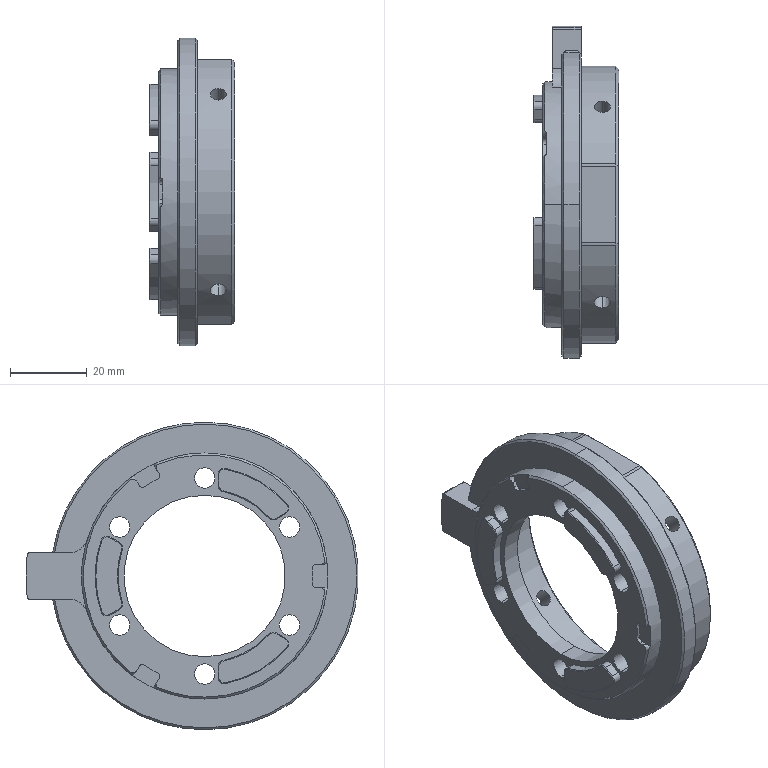NC program | NX | posted with a generic post | part box 22.3 x 86.5 x 80 mm
Lines 951 to 2662 of 3025, first 1570 of 1708 lines:
(FLOOR_WALL_2_COPY_COPY_COPY , TOOL : D2)
N1870 T18 M6
N1872 G54
N1874 G17 G0 G90 X17.592 Y-29.095 S9500 M3
N1876 G43 Z30. H18
N1878 Z-1.643
N1880 G94 G1 Z-2.643 F1000.
N1882 X16.699 Y-28.58
N1884 G3 X16.499 Y-28.58 R0.2
N1886 G2 X14.117 Y-29.828 R33.
N1888 G1 X14.015 Y-28.558
N1890 X13.875 Y-28.11
N1892 X13.705 Y-27.738
N1894 X12.733 Y-26.055
N1896 G3 X16.198 Y-24.055 R29.
N1898 G1 X17.177 Y-25.752
N1900 X17.559 Y-26.254
N1902 X17.669 Y-26.351
N1904 X17.916 Y-26.566
N1906 X18.799 Y-27.122
N1908 G2 X16.499 Y-28.58 R33.
N1910 G1 X15.999 Y-27.714
N1912 X15.997
N1914 G2 X14.976 Y-28.279 R32.
N1916 G1 X14.811 Y-27.751
N1918 X14.595 Y-27.279
N1920 X14.126 Y-26.466
N1922 G3 X15.858 Y-25.466 R30.
N1924 G1 X16.343 Y-26.307
N1926 X16.824 Y-26.94
N1928 X17.011 Y-27.104
N1930 G2 X15.999 Y-27.714 R32.
N1932 G1 X15.499 Y-26.848
N1934 G3 X15.399 Y-27.021 R0.2
N1936 G1 X16.834 Y-29.54
N1938 Z-1.643
N1940 G0 X17.592 Y-29.095 Z-1.786
N1942 G1 Z-2.786
N1944 X16.699 Y-28.58
N1946 G3 X16.499 Y-28.58 R0.2
N1948 G2 X14.117 Y-29.828 R33.
N1950 G1 X14.015 Y-28.558
N1952 X13.875 Y-28.11
N1954 X13.705 Y-27.738
N1956 X12.733 Y-26.055
N1958 G3 X16.198 Y-24.055 R29.
N1960 G1 X17.177 Y-25.752
N1962 X17.559 Y-26.254
N1964 X17.669 Y-26.351
N1966 X17.916 Y-26.566
N1968 X18.799 Y-27.122
N1970 G2 X16.499 Y-28.58 R33.
N1972 G1 X15.999 Y-27.714
N1974 X15.997
N1976 G2 X14.976 Y-28.279 R32.
N1978 G1 X14.811 Y-27.751
N1980 X14.595 Y-27.279
N1982 X14.126 Y-26.466
N1984 G3 X15.858 Y-25.466 R30.
N1986 G1 X16.343 Y-26.307
N1988 X16.824 Y-26.94
N1990 X17.011 Y-27.104
N1992 G2 X15.999 Y-27.714 R32.
N1994 G1 X15.499 Y-26.848
N1996 G3 X15.399 Y-27.021 R0.2
N1998 G1 X16.834 Y-29.54
N2000 Z-1.786
N2002 G0 X17.592 Y-29.095 Z-1.929
N2004 G1 Z-2.929
N2006 X16.699 Y-28.58
N2008 G3 X16.499 Y-28.58 R0.2
N2010 G2 X14.117 Y-29.828 R33.
N2012 G1 X14.015 Y-28.558
N2014 X13.875 Y-28.11
N2016 X13.705 Y-27.738
N2018 X12.733 Y-26.055
N2020 G3 X16.198 Y-24.055 R29.
N2022 G1 X17.177 Y-25.752
N2024 X17.559 Y-26.254
N2026 X17.669 Y-26.351
N2028 X17.916 Y-26.566
N2030 X18.799 Y-27.122
N2032 G2 X16.499 Y-28.58 R33.
N2034 G1 X15.999 Y-27.714
N2036 X15.997
N2038 G2 X14.976 Y-28.279 R32.
N2040 G1 X14.811 Y-27.751
N2042 X14.595 Y-27.279
N2044 X14.126 Y-26.466
N2046 G3 X15.858 Y-25.466 R30.
N2048 G1 X16.343 Y-26.307
N2050 X16.824 Y-26.94
N2052 X17.011 Y-27.104
N2054 G2 X15.999 Y-27.714 R32.
N2056 G1 X15.499 Y-26.848
N2058 G3 X15.399 Y-27.021 R0.2
N2060 G1 X16.834 Y-29.54
N2062 Z-1.929
N2064 G0 X17.592 Y-29.095 Z-2.071
N2066 G1 Z-3.071
N2068 X16.699 Y-28.58
N2070 G3 X16.499 Y-28.58 R0.2
N2072 G2 X14.117 Y-29.828 R33.
N2074 G1 X14.015 Y-28.558
N2076 X13.875 Y-28.11
N2078 X13.705 Y-27.738
N2080 X12.733 Y-26.055
N2082 G3 X16.198 Y-24.055 R29.
N2084 G1 X17.177 Y-25.752
N2086 X17.559 Y-26.254
N2088 X17.669 Y-26.351
N2090 X17.916 Y-26.566
N2092 X18.799 Y-27.122
N2094 G2 X16.499 Y-28.58 R33.
N2096 G1 X15.999 Y-27.714
N2098 X15.997
N2100 G2 X14.976 Y-28.279 R32.
N2102 G1 X14.811 Y-27.751
N2104 X14.595 Y-27.279
N2106 X14.126 Y-26.466
N2108 G3 X15.858 Y-25.466 R30.
N2110 G1 X16.343 Y-26.307
N2112 X16.824 Y-26.94
N2114 X17.011 Y-27.104
N2116 G2 X15.999 Y-27.714 R32.
N2118 G1 X15.499 Y-26.848
N2120 G3 X15.399 Y-27.021 R0.2
N2122 G1 X16.834 Y-29.54
N2124 Z-2.071
N2126 G0 X17.592 Y-29.095 Z-2.214
N2128 G1 Z-3.214
N2130 X16.699 Y-28.58
N2132 G3 X16.499 Y-28.58 R0.2
N2134 G2 X14.117 Y-29.828 R33.
N2136 G1 X14.015 Y-28.558
N2138 X13.875 Y-28.11
N2140 X13.705 Y-27.738
N2142 X12.733 Y-26.055
N2144 G3 X16.198 Y-24.055 R29.
N2146 G1 X17.177 Y-25.752
N2148 X17.559 Y-26.254
N2150 X17.669 Y-26.351
N2152 X17.916 Y-26.566
N2154 X18.799 Y-27.122
N2156 G2 X16.499 Y-28.58 R33.
N2158 G1 X15.999 Y-27.714
N2160 X15.997
N2162 G2 X14.976 Y-28.279 R32.
N2164 G1 X14.811 Y-27.751
N2166 X14.595 Y-27.279
N2168 X14.126 Y-26.466
N2170 G3 X15.858 Y-25.466 R30.
N2172 G1 X16.343 Y-26.307
N2174 X16.824 Y-26.94
N2176 X17.011 Y-27.104
N2178 G2 X15.999 Y-27.714 R32.
N2180 G1 X15.499 Y-26.848
N2182 G3 X15.399 Y-27.021 R0.2
N2184 G1 X16.834 Y-29.54
N2186 Z-2.214
N2188 G0 X17.592 Y-29.095 Z-2.357
N2190 G1 Z-3.357
N2192 X16.699 Y-28.58
N2194 G3 X16.499 Y-28.58 R0.2
N2196 G2 X14.117 Y-29.828 R33.
N2198 G1 X14.015 Y-28.558
N2200 X13.875 Y-28.11
N2202 X13.705 Y-27.738
N2204 X12.733 Y-26.055
N2206 G3 X16.198 Y-24.055 R29.
N2208 G1 X17.177 Y-25.752
N2210 X17.559 Y-26.254
N2212 X17.669 Y-26.351
N2214 X17.916 Y-26.566
N2216 X18.799 Y-27.122
N2218 G2 X16.499 Y-28.58 R33.
N2220 G1 X15.999 Y-27.714
N2222 X15.997
N2224 G2 X14.976 Y-28.279 R32.
N2226 G1 X14.811 Y-27.751
N2228 X14.595 Y-27.279
N2230 X14.126 Y-26.466
N2232 G3 X15.858 Y-25.466 R30.
N2234 G1 X16.343 Y-26.307
N2236 X16.824 Y-26.94
N2238 X17.011 Y-27.104
N2240 G2 X15.999 Y-27.714 R32.
N2242 G1 X15.499 Y-26.848
N2244 G3 X15.399 Y-27.021 R0.2
N2246 G1 X16.834 Y-29.54
N2248 Z-2.357
N2250 G0 X17.592 Y-29.095 Z-2.5
N2252 G1 Z-3.5
N2254 X16.699 Y-28.58
N2256 G3 X16.499 Y-28.58 R0.2
N2258 G2 X14.117 Y-29.828 R33.
N2260 G1 X14.015 Y-28.558
N2262 X13.875 Y-28.11
N2264 X13.705 Y-27.738
N2266 X12.733 Y-26.055
N2268 G3 X16.198 Y-24.055 R29.
N2270 G1 X17.177 Y-25.752
N2272 X17.559 Y-26.254
N2274 X17.669 Y-26.351
N2276 X17.916 Y-26.566
N2278 X18.799 Y-27.122
N2280 G2 X16.499 Y-28.58 R33.
N2282 G1 X15.999 Y-27.714
N2284 X15.997
N2286 G2 X14.976 Y-28.279 R32.
N2288 G1 X14.811 Y-27.751
N2290 X14.595 Y-27.279
N2292 X14.126 Y-26.466
N2294 G3 X15.858 Y-25.466 R30.
N2296 G1 X16.343 Y-26.307
N2298 X16.824 Y-26.94
N2300 X17.011 Y-27.104
N2302 G2 X15.999 Y-27.714 R32.
N2304 G1 X15.499 Y-26.848
N2306 G3 X15.399 Y-27.021 R0.2
N2308 G1 X16.834 Y-29.54
N2310 Z-2.5
N2312 G0 Z30.
N2314 X16.401 Y29.782
N2316 Z-1.643
N2318 G1 Z-2.643
N2320 Y28.751
N2322 G3 X16.501 Y28.578 R0.2
N2324 G2 X18.774 Y27.139 R33.
N2326 G1 X17.725 Y26.417
N2328 X17.406 Y26.071
N2330 X17.169 Y25.738
N2332 X16.198 Y24.055
N2334 G3 X12.733 Y26.055 R29.
N2336 G1 X13.713 Y27.752
N2338 X13.957 Y28.334
N2340 X13.986 Y28.478
N2342 X14.049 Y28.799
N2344 X14.089 Y29.841
N2346 G2 X16.501 Y28.578 R33.
N2348 G1 X16.001 Y27.712
N2350 X16.003 Y27.711
N2352 G2 X17.003 Y27.109 R32.
N2354 G1 X16.628 Y26.702
N2356 X16.327 Y26.279
N2358 X15.858 Y25.466
N2360 G3 X14.126 Y26.466 R30.
N2362 G1 X14.611 Y27.307
N2364 X14.919 Y28.041
N2366 X14.967 Y28.284
N2368 G2 X16.001 Y27.712 R32.
N2370 G1 X15.501 Y26.846
N2372 G3 X15.701 Y26.846 R0.2
N2374 G1 X17.165 Y29.349
N2376 Z-1.643
N2378 G0 X16.401 Y29.782 Z-1.786
N2380 G1 Z-2.786
N2382 Y28.751
N2384 G3 X16.501 Y28.578 R0.2
N2386 G2 X18.774 Y27.139 R33.
N2388 G1 X17.725 Y26.417
N2390 X17.406 Y26.071
N2392 X17.169 Y25.738
N2394 X16.198 Y24.055
N2396 G3 X12.733 Y26.055 R29.
N2398 G1 X13.713 Y27.752
N2400 X13.957 Y28.334
N2402 X13.986 Y28.478
N2404 X14.049 Y28.799
N2406 X14.089 Y29.841
N2408 G2 X16.501 Y28.578 R33.
N2410 G1 X16.001 Y27.712
N2412 X16.003 Y27.711
N2414 G2 X17.003 Y27.109 R32.
N2416 G1 X16.628 Y26.702
N2418 X16.327 Y26.279
N2420 X15.858 Y25.466
N2422 G3 X14.126 Y26.466 R30.
N2424 G1 X14.611 Y27.307
N2426 X14.919 Y28.041
N2428 X14.967 Y28.284
N2430 G2 X16.001 Y27.712 R32.
N2432 G1 X15.501 Y26.846
N2434 G3 X15.701 Y26.846 R0.2
N2436 G1 X17.165 Y29.349
N2438 Z-1.786
N2440 G0 X16.401 Y29.782 Z-1.929
N2442 G1 Z-2.929
N2444 Y28.751
N2446 G3 X16.501 Y28.578 R0.2
N2448 G2 X18.774 Y27.139 R33.
N2450 G1 X17.725 Y26.417
N2452 X17.406 Y26.071
N2454 X17.169 Y25.738
N2456 X16.198 Y24.055
N2458 G3 X12.733 Y26.055 R29.
N2460 G1 X13.713 Y27.752
N2462 X13.957 Y28.334
N2464 X13.986 Y28.478
N2466 X14.049 Y28.799
N2468 X14.089 Y29.841
N2470 G2 X16.501 Y28.578 R33.
N2472 G1 X16.001 Y27.712
N2474 X16.003 Y27.711
N2476 G2 X17.003 Y27.109 R32.
N2478 G1 X16.628 Y26.702
N2480 X16.327 Y26.279
N2482 X15.858 Y25.466
N2484 G3 X14.126 Y26.466 R30.
N2486 G1 X14.611 Y27.307
N2488 X14.919 Y28.041
N2490 X14.967 Y28.284
N2492 G2 X16.001 Y27.712 R32.
N2494 G1 X15.501 Y26.846
N2496 G3 X15.701 Y26.846 R0.2
N2498 G1 X17.165 Y29.349
N2500 Z-1.929
N2502 G0 X16.401 Y29.782 Z-2.071
N2504 G1 Z-3.071
N2506 Y28.751
N2508 G3 X16.501 Y28.578 R0.2
N2510 G2 X18.774 Y27.139 R33.
N2512 G1 X17.725 Y26.417
N2514 X17.406 Y26.071
N2516 X17.169 Y25.738
N2518 X16.198 Y24.055
N2520 G3 X12.733 Y26.055 R29.
N2522 G1 X13.713 Y27.752
N2524 X13.957 Y28.334
N2526 X13.986 Y28.478
N2528 X14.049 Y28.799
N2530 X14.089 Y29.841
N2532 G2 X16.501 Y28.578 R33.
N2534 G1 X16.001 Y27.712
N2536 X16.003 Y27.711
N2538 G2 X17.003 Y27.109 R32.
N2540 G1 X16.628 Y26.702
N2542 X16.327 Y26.279
N2544 X15.858 Y25.466
N2546 G3 X14.126 Y26.466 R30.
N2548 G1 X14.611 Y27.307
N2550 X14.919 Y28.041
N2552 X14.967 Y28.284
N2554 G2 X16.001 Y27.712 R32.
N2556 G1 X15.501 Y26.846
N2558 G3 X15.701 Y26.846 R0.2
N2560 G1 X17.165 Y29.349
N2562 Z-2.071
N2564 G0 X16.401 Y29.782 Z-2.214
N2566 G1 Z-3.214
N2568 Y28.751
N2570 G3 X16.501 Y28.578 R0.2
N2572 G2 X18.774 Y27.139 R33.
N2574 G1 X17.725 Y26.417
N2576 X17.406 Y26.071
N2578 X17.169 Y25.738
N2580 X16.198 Y24.055
N2582 G3 X12.733 Y26.055 R29.
N2584 G1 X13.713 Y27.752
N2586 X13.957 Y28.334
N2588 X13.986 Y28.478
N2590 X14.049 Y28.799
N2592 X14.089 Y29.841
N2594 G2 X16.501 Y28.578 R33.
N2596 G1 X16.001 Y27.712
N2598 X16.003 Y27.711
N2600 G2 X17.003 Y27.109 R32.
N2602 G1 X16.628 Y26.702
N2604 X16.327 Y26.279
N2606 X15.858 Y25.466
N2608 G3 X14.126 Y26.466 R30.
N2610 G1 X14.611 Y27.307
N2612 X14.919 Y28.041
N2614 X14.967 Y28.284
N2616 G2 X16.001 Y27.712 R32.
N2618 G1 X15.501 Y26.846
N2620 G3 X15.701 Y26.846 R0.2
N2622 G1 X17.165 Y29.349
N2624 Z-2.214
N2626 G0 X16.401 Y29.782 Z-2.357
N2628 G1 Z-3.357
N2630 Y28.751
N2632 G3 X16.501 Y28.578 R0.2
N2634 G2 X18.774 Y27.139 R33.
N2636 G1 X17.725 Y26.417
N2638 X17.406 Y26.071
N2640 X17.169 Y25.738
N2642 X16.198 Y24.055
N2644 G3 X12.733 Y26.055 R29.
N2646 G1 X13.713 Y27.752
N2648 X13.957 Y28.334
N2650 X13.986 Y28.478
N2652 X14.049 Y28.799
N2654 X14.089 Y29.841
N2656 G2 X16.501 Y28.578 R33.
N2658 G1 X16.001 Y27.712
N2660 X16.003 Y27.711
N2662 G2 X17.003 Y27.109 R32.
N2664 G1 X16.628 Y26.702
N2666 X16.327 Y26.279
N2668 X15.858 Y25.466
N2670 G3 X14.126 Y26.466 R30.
N2672 G1 X14.611 Y27.307
N2674 X14.919 Y28.041
N2676 X14.967 Y28.284
N2678 G2 X16.001 Y27.712 R32.
N2680 G1 X15.501 Y26.846
N2682 G3 X15.701 Y26.846 R0.2
N2684 G1 X17.165 Y29.349
N2686 Z-2.357
N2688 G0 X16.401 Y29.782 Z-2.5
N2690 G1 Z-3.5
N2692 Y28.751
N2694 G3 X16.501 Y28.578 R0.2
N2696 G2 X18.774 Y27.139 R33.
N2698 G1 X17.725 Y26.417
N2700 X17.406 Y26.071
N2702 X17.169 Y25.738
N2704 X16.198 Y24.055
N2706 G3 X12.733 Y26.055 R29.
N2708 G1 X13.713 Y27.752
N2710 X13.957 Y28.334
N2712 X13.986 Y28.478
N2714 X14.049 Y28.799
N2716 X14.089 Y29.841
N2718 G2 X16.501 Y28.578 R33.
N2720 G1 X16.001 Y27.712
N2722 X16.003 Y27.711
N2724 G2 X17.003 Y27.109 R32.
N2726 G1 X16.628 Y26.702
N2728 X16.327 Y26.279
N2730 X15.858 Y25.466
N2732 G3 X14.126 Y26.466 R30.
N2734 G1 X14.611 Y27.307
N2736 X14.919 Y28.041
N2738 X14.967 Y28.284
N2740 G2 X16.001 Y27.712 R32.
N2742 G1 X15.501 Y26.846
N2744 G3 X15.701 Y26.846 R0.2
N2746 G1 X17.165 Y29.349
N2748 Z-2.5
N2750 G0 Z30.
N2752 X-33.993 Y-0.687
N2754 Z-1.643
N2756 G1 Z-2.643
N2758 X-33.1 Y-0.172
N2760 G3 X-33. Y0.002 R0.2
N2762 G2 X-32.89 Y2.689 R33.
N2764 G1 X-31.74 Y2.142
N2766 X-31.281 Y2.038
N2768 X-30.874 Y2.
N2770 X-28.931
N2772 G3 X-28.931 Y-2. R29.
N2774 G1 X-30.891
N2776 X-31.517 Y-2.079
N2778 X-31.655 Y-2.127
N2780 X-31.965 Y-2.233
N2782 X-32.888 Y-2.719
N2784 G2 X-33. Y0.002 R33.
N2786 G1 X-32.
N2788 Y0.003
N2790 G2 X-31.979 Y1.17 R32.
N2792 G1 X-31.439 Y1.049
N2794 X-30.921 Y1.
N2796 X-29.983
N2798 G3 X-29.983 Y-1. R30.
N2800 G1 X-30.954
N2802 X-31.743 Y-1.1
N2804 X-31.978 Y-1.18
N2806 G2 X-32. Y0.002 R32.
N2808 G1 X-31. Y0.001
N2810 G3 X-31.1 Y0.175 R0.2
N2812 G1 X-33.999 Y0.191
N2814 Z-1.643
N2816 G0 X-33.993 Y-0.687 Z-1.786
N2818 G1 Z-2.786
N2820 X-33.1 Y-0.172
N2822 G3 X-33. Y0.002 R0.2
N2824 G2 X-32.89 Y2.689 R33.
N2826 G1 X-31.74 Y2.142
N2828 X-31.281 Y2.038
N2830 X-30.874 Y2.
N2832 X-28.931
N2834 G3 X-28.931 Y-2. R29.
N2836 G1 X-30.891
N2838 X-31.517 Y-2.079
N2840 X-31.655 Y-2.127
N2842 X-31.965 Y-2.233
N2844 X-32.888 Y-2.719
N2846 G2 X-33. Y0.002 R33.
N2848 G1 X-32.
N2850 Y0.003
N2852 G2 X-31.979 Y1.17 R32.
N2854 G1 X-31.439 Y1.049
N2856 X-30.921 Y1.
N2858 X-29.983
N2860 G3 X-29.983 Y-1. R30.
N2862 G1 X-30.954
N2864 X-31.743 Y-1.1
N2866 X-31.978 Y-1.18
N2868 G2 X-32. Y0.002 R32.
N2870 G1 X-31. Y0.001
N2872 G3 X-31.1 Y0.175 R0.2
N2874 G1 X-33.999 Y0.191
N2876 Z-1.786
N2878 G0 X-33.993 Y-0.687 Z-1.929
N2880 G1 Z-2.929
N2882 X-33.1 Y-0.172
N2884 G3 X-33. Y0.002 R0.2
N2886 G2 X-32.89 Y2.689 R33.
N2888 G1 X-31.74 Y2.142
N2890 X-31.281 Y2.038
N2892 X-30.874 Y2.
N2894 X-28.931
N2896 G3 X-28.931 Y-2. R29.
N2898 G1 X-30.891
N2900 X-31.517 Y-2.079
N2902 X-31.655 Y-2.127
N2904 X-31.965 Y-2.233
N2906 X-32.888 Y-2.719
N2908 G2 X-33. Y0.002 R33.
N2910 G1 X-32.
N2912 Y0.003
N2914 G2 X-31.979 Y1.17 R32.
N2916 G1 X-31.439 Y1.049
N2918 X-30.921 Y1.
N2920 X-29.983
N2922 G3 X-29.983 Y-1. R30.
N2924 G1 X-30.954
N2926 X-31.743 Y-1.1
N2928 X-31.978 Y-1.18
N2930 G2 X-32. Y0.002 R32.
N2932 G1 X-31. Y0.001
N2934 G3 X-31.1 Y0.175 R0.2
N2936 G1 X-33.999 Y0.191
N2938 Z-1.929
N2940 G0 X-33.993 Y-0.687 Z-2.071
N2942 G1 Z-3.071
N2944 X-33.1 Y-0.172
N2946 G3 X-33. Y0.002 R0.2
N2948 G2 X-32.89 Y2.689 R33.
N2950 G1 X-31.74 Y2.142
N2952 X-31.281 Y2.038
N2954 X-30.874 Y2.
N2956 X-28.931
N2958 G3 X-28.931 Y-2. R29.
N2960 G1 X-30.891
N2962 X-31.517 Y-2.079
N2964 X-31.655 Y-2.127
N2966 X-31.965 Y-2.233
N2968 X-32.888 Y-2.719
N2970 G2 X-33. Y0.002 R33.
N2972 G1 X-32.
N2974 Y0.003
N2976 G2 X-31.979 Y1.17 R32.
N2978 G1 X-31.439 Y1.049
N2980 X-30.921 Y1.
N2982 X-29.983
N2984 G3 X-29.983 Y-1. R30.
N2986 G1 X-30.954
N2988 X-31.743 Y-1.1
N2990 X-31.978 Y-1.18
N2992 G2 X-32. Y0.002 R32.
N2994 G1 X-31. Y0.001
N2996 G3 X-31.1 Y0.175 R0.2
N2998 G1 X-33.999 Y0.191
N3000 Z-2.071
N3002 G0 X-33.993 Y-0.687 Z-2.214
N3004 G1 Z-3.214
N3006 X-33.1 Y-0.172
N3008 G3 X-33. Y0.002 R0.2
N3010 G2 X-32.89 Y2.689 R33.
N3012 G1 X-31.74 Y2.142
N3014 X-31.281 Y2.038
N3016 X-30.874 Y2.
N3018 X-28.931
N3020 G3 X-28.931 Y-2. R29.
N3022 G1 X-30.891
N3024 X-31.517 Y-2.079
N3026 X-31.655 Y-2.127
N3028 X-31.965 Y-2.233
N3030 X-32.888 Y-2.719
N3032 G2 X-33. Y0.002 R33.
N3034 G1 X-32.
N3036 Y0.003
N3038 G2 X-31.979 Y1.17 R32.
N3040 G1 X-31.439 Y1.049
N3042 X-30.921 Y1.
N3044 X-29.983
N3046 G3 X-29.983 Y-1. R30.
N3048 G1 X-30.954
N3050 X-31.743 Y-1.1
N3052 X-31.978 Y-1.18
N3054 G2 X-32. Y0.002 R32.
N3056 G1 X-31. Y0.001
N3058 G3 X-31.1 Y0.175 R0.2
N3060 G1 X-33.999 Y0.191
N3062 Z-2.214
N3064 G0 X-33.993 Y-0.687 Z-2.357
N3066 G1 Z-3.357
N3068 X-33.1 Y-0.172
N3070 G3 X-33. Y0.002 R0.2
N3072 G2 X-32.89 Y2.689 R33.
N3074 G1 X-31.74 Y2.142
N3076 X-31.281 Y2.038
N3078 X-30.874 Y2.
N3080 X-28.931
N3082 G3 X-28.931 Y-2. R29.
N3084 G1 X-30.891
N3086 X-31.517 Y-2.079
N3088 X-31.655 Y-2.127
N3090 X-31.965 Y-2.233
N3092 X-32.888 Y-2.719
N3094 G2 X-33. Y0.002 R33.
N3096 G1 X-32.
N3098 Y0.003
N3100 G2 X-31.979 Y1.17 R32.
N3102 G1 X-31.439 Y1.049
N3104 X-30.921 Y1.
N3106 X-29.983
N3108 G3 X-29.983 Y-1. R30.
N3110 G1 X-30.954
N3112 X-31.743 Y-1.1
N3114 X-31.978 Y-1.18
N3116 G2 X-32. Y0.002 R32.
N3118 G1 X-31. Y0.001
N3120 G3 X-31.1 Y0.175 R0.2
N3122 G1 X-33.999 Y0.191
N3124 Z-2.357
N3126 G0 X-33.993 Y-0.687 Z-2.5
N3128 G1 Z-3.5
N3130 X-33.1 Y-0.172
N3132 G3 X-33. Y0.002 R0.2
N3134 G2 X-32.89 Y2.689 R33.
N3136 G1 X-31.74 Y2.142
N3138 X-31.281 Y2.038
N3140 X-30.874 Y2.
N3142 X-28.931
N3144 G3 X-28.931 Y-2. R29.
N3146 G1 X-30.891
N3148 X-31.517 Y-2.079
N3150 X-31.655 Y-2.127
N3152 X-31.965 Y-2.233
N3154 X-32.888 Y-2.719
N3156 G2 X-33. Y0.002 R33.
N3158 G1 X-32.
N3160 Y0.003
N3162 G2 X-31.979 Y1.17 R32.
N3164 G1 X-31.439 Y1.049
N3166 X-30.921 Y1.
N3168 X-29.983
N3170 G3 X-29.983 Y-1. R30.
N3172 G1 X-30.954
N3174 X-31.743 Y-1.1
N3176 X-31.978 Y-1.18
N3178 G2 X-32. Y0.002 R32.
N3180 G1 X-31. Y0.001
N3182 G3 X-31.1 Y0.175 R0.2
N3184 G1 X-33.999 Y0.191
N3186 Z-2.5
N3188 G0 Z30.
(ZLEVEL_PROFILE_1_COPY , TOOL : D2)
N3190 X13.293 Y-26.223
N3192 Z-1.035
N3194 G1 Z-2.535 F1500.
N3196 X12.905 Y-26.156
N3198 G3 X12.907 Y-26.356 R0.2
N3200 G2 X13.255 Y-26.971 R17.468
N3202 X13.543 Y-28.664 R2.678
N3204 X12.415 Y-30.075 R1.83
N3206 G1 X11.91 Y-30.277
N3208 Y-30.315 Z-2.571
N3210 X12.464 Y-30.09
N3212 G3 X13.534 Y-28.822 R1.779
N3214 X13.308 Y-27.066 R2.629
N3216 G1 X12.907 Y-26.356
N3218 Z-2.606
N3220 X13.273 Y-27.001
N3222 G2 X13.555 Y-28.835 R2.609
N3224 X12.508 Y-30.111 R1.801
N3226 G1 X11.91 Y-30.353
N3228 Y-30.391 Z-2.641
N3230 X12.508 Y-30.149
N3232 G3 X13.578 Y-28.84 R1.804
N3234 X13.312 Y-27.066 R2.651
N3236 G1 X12.907 Y-26.356
N3238 Z-2.676
N3240 X13.315 Y-27.066
N3242 G2 X13.624 Y-28.723 R2.713
N3244 X12.486 Y-30.197 R1.853
N3246 G1 X12.109 Y-30.35
N3248 Y-30.388 Z-2.712
N3250 X12.508 Y-30.226
N3252 G3 X13.655 Y-28.643 R1.838
N3254 X13.316 Y-27.066 R2.772
N3256 G1 X12.907 Y-26.356
N3258 Z-2.747
N3260 G2 X13.413 Y-27.264 R14.43
N3262 X13.603 Y-29.041 R2.535
N3264 X12.649 Y-30.2 R1.779
N3266 G1 X12.608 Y-30.219
N3268 X12.133 Y-30.416
N3270 X12.109 Y-30.464 Z-2.782
N3272 G3 X12.713 Y-30.204 R4.238
N3274 X13.669 Y-28.877 R1.832
N3276 X13.416 Y-27.264 R2.616
N3278 X12.907 Y-26.356 R18.367
N3280 G1 X12.976 Y-26.475 Z-2.818
N3282 G2 X13.419 Y-27.264 R17.197
N3284 X13.663 Y-29.011 R2.591
N3286 X12.568 Y-30.317 R1.813
N3288 G1 X12.109 Y-30.502
N3290 Y-30.54 Z-2.853
N3292 X12.577 Y-30.351
N3294 G3 X13.707 Y-28.926 R1.839
N3296 X13.422 Y-27.264 R2.661
N3298 X12.976 Y-26.475 R23.63
N3300 G1 Z-2.888
N3302 X13.425 Y-27.264
N3304 X13.506 Y-27.424
N3306 G2 X13.713 Y-29.015 R2.653
N3308 X12.605 Y-30.378 R1.815
N3310 G1 X12.109 Y-30.578
N3312 X12.115 Y-30.613 Z-2.924
N3314 X12.656 Y-30.392
N3316 G3 X13.616 Y-29.419 R1.743
N3318 X13.753 Y-28.249 R2.294
N3320 X13.428 Y-27.264 R2.927
N3322 G1 X12.976 Y-26.475
N3324 Z-2.959
N3326 X13.43 Y-27.264
N3328 G2 X13.705 Y-27.942 R3.263
N3330 X13.714 Y-29.219 R2.526
N3332 X12.804 Y-30.361 R1.773
N3334 X12.211 Y-30.613 R4.489
N3336 G1 X12.16 Y-30.653 Z-2.976
N3338 X12.109 Y-30.692 Z-2.994
N3340 X12.708 Y-30.449
N3342 G3 X13.705 Y-29.342 R1.786
N3344 X13.705 Y-27.912 R2.486
N3346 X13.431 Y-27.264 R3.303
N3348 G1 X12.976 Y-26.475
N3350 Z-3.029
N3352 X13.506 Y-27.402
N3354 X13.531 Y-27.461
N3356 X13.585 Y-27.576
N3358 G2 X13.757 Y-29.248 R2.557
N3360 X12.748 Y-30.46 R1.766
N3362 G1 X12.303 Y-30.655
N3364 X12.322 Y-30.685 Z-3.065
N3366 X12.755 Y-30.497
N3368 G3 X13.78 Y-29.261 R1.78
N3370 X13.615 Y-27.639 R2.551
N3372 G1 X13.506 Y-27.398
N3374 X13.107 Y-26.701
N3376 Z-3.1
N3378 X13.506 Y-27.395
N3380 X13.603 Y-27.598
N3382 G2 X13.806 Y-29.258 R2.602
N3384 X12.767 Y-30.531 R1.784
N3386 G1 X12.34 Y-30.715
N3388 X12.359 Y-30.745 Z-3.135
N3390 G3 X12.897 Y-30.509 R3.901
N3392 X13.863 Y-29.081 R1.842
N3394 X13.54 Y-27.461 R2.759
N3396 G1 X13.506 Y-27.393
N3398 X13.107 Y-26.701
N3400 Z-3.17
N3402 X13.543 Y-27.461
N3404 G2 X13.902 Y-28.84 R2.931
N3406 X13.107 Y-30.432 R1.944
N3408 X12.377 Y-30.776 R4.073
N3410 G1 X12.396 Y-30.807 Z-3.206
N3412 G3 X13.306 Y-30.318 R2.886
N3414 X13.912 Y-28.643 R2.032
N3416 X13.544 Y-27.461 R3.002
N3418 G1 X13.107 Y-26.701
N3420 Z-3.241
N3422 G2 X13.643 Y-27.658 R16.017
N3424 X13.903 Y-29.271 R2.634
N3426 X12.931 Y-30.613 R1.825
N3428 X12.436 Y-30.827 R4.263
N3430 G1 X12.479 Y-30.848 Z-3.276
N3432 X13.016 Y-30.611
N3434 G3 X13.906 Y-29.367 R1.809
N3436 X13.646 Y-27.658 R2.626
N3438 X13.204 Y-26.869 R16.196
N3440 G1 Z-3.311
N3442 G2 X13.65 Y-27.658 R20.176
N3444 X13.952 Y-29.234 R2.687
N3446 X12.586 Y-30.841 R1.894
N3448 G1 X12.67 Y-30.821 Z-3.323
N3450 X12.753 Y-30.799 Z-3.335
N3452 X12.835 Y-30.774 Z-3.347
N3454 G3 X13.941 Y-29.431 R1.801
N3456 X13.705 Y-27.754 R2.705
N3458 X13.204 Y-26.869 R29.664
N3460 G1 Z-3.382
N3462 X13.656 Y-27.658
N3464 X13.705 Y-27.75
N3466 G2 X13.965 Y-29.431 R2.677
N3468 X13.169 Y-30.644 R1.839
N3470 G1 X13.239 Y-30.614 Z-3.394
N3472 X13.307 Y-30.578 Z-3.406
N3474 X13.368 Y-30.535 Z-3.417
N3476 G3 X13.989 Y-29.431 R1.827
N3478 X13.705 Y-27.747 R2.675
N3480 G1 X13.658 Y-27.658
N3482 X13.204 Y-26.869
N3484 Z-3.453
N3486 X13.659 Y-27.658
N3488 X13.705 Y-27.744
N3490 G2 X14.038 Y-29.234 R2.746
N3492 X13.524 Y-30.443 R1.972
N3494 G1 X13.582 Y-30.406 Z-3.472
N3496 X13.634 Y-30.365 Z-3.49
N3498 G3 X14.06 Y-29.234 R1.973
N3500 X13.705 Y-27.74 R2.754
N3502 G1 X13.659 Y-27.658
N3504 X13.317 Y-27.066
N3506 Z-3.5
N3508 X13.659 Y-27.658
N3510 X13.705 Y-27.739
N3512 G2 X14.064 Y-29.234 R2.76
N3514 X13.655 Y-30.35 R1.984
N3516 G3 X13.629 Y-30.548 R0.2
N3518 G1 X13.745 Y-30.83
N3520 Z-2.
N3522 G0 Z30.
N3524 X20.79 Y-25.544
N3526 Z-1.035
N3528 G1 Z-2.535
N3530 X20.248 Y-25.497
N3532 X20.211 Y-25.49
N3534 X20.176 Y-25.506
N3536 X20.157 Y-25.539
N3538 X20.15 Y-25.549
N3540 X19.706 Y-25.884
N3542 X19.689 Y-25.896
N3544 G2 X17.894 Y-25.997 R1.851
N3546 X16.697 Y-24.916 R2.733
N3548 G1 X16.343 Y-24.308
N3550 Z-2.571
N3552 X16.686 Y-24.899
N3554 G3 X17.94 Y-26.041 R2.752
N3556 X19.71 Y-25.918 R1.866
N3558 X20.17 Y-25.574 R3.709
N3560 G1 X20.182 Y-25.591 Z-2.588
N3562 X20.191 Y-25.602 Z-2.606
N3564 G2 X19.489 Y-26.087 R3.67
N3566 X17.894 Y-26.043 R1.893
N3568 X16.813 Y-25.096 R2.664
N3570 X16.343 Y-24.308 R15.612
N3572 G1 Z-2.641
N3574 G3 X16.81 Y-25.096 R18.778
N3576 X17.894 Y-26.066 R2.68
N3578 X19.489 Y-26.125 R1.899
N3580 X20.212 Y-25.631 R3.572
N3582 G1 X20.224 Y-25.666 Z-2.676
N3584 G2 X19.706 Y-26.045 R3.413
N3586 X17.92 Y-26.102 R1.843
N3588 G1 X17.88 Y-26.081
N3590 G2 X16.807 Y-25.096 R2.697
N3592 G1 X16.343 Y-24.308
N3594 Z-2.712
N3596 X16.804 Y-25.096
N3598 G3 X17.838 Y-26.081 R2.727
N3600 G1 X17.942 Y-26.135
N3602 G3 X19.702 Y-26.089 R1.836
N3604 X20.252 Y-25.689 R3.297
N3606 G1 X20.263 Y-25.708 Z-2.729
N3608 X20.27 Y-25.72 Z-2.747
N3610 G2 X19.489 Y-26.241 R3.151
N3612 X17.894 Y-26.131 R1.924
N3614 X16.801 Y-25.096 R2.754
N3616 G1 X16.343 Y-24.308
N3618 Z-2.782
N3620 X16.799 Y-25.096
N3622 G3 X18.095 Y-26.248 R2.755
N3624 X19.73 Y-26.155 R1.832
N3626 X20.287 Y-25.751 R3.233
N3628 G1 X20.301 Y-25.785 Z-2.818
N3630 G2 X19.842 Y-26.129 R4.355
N3632 X18.118 Y-26.282 R1.843
N3634 X16.927 Y-25.293 R2.685
N3636 X16.343 Y-24.308 R20.422
N3638 G1 X16.457 Y-24.505 Z-2.853
N3640 G3 X16.896 Y-25.25 R21.125
N3642 X18.125 Y-26.306 R2.674
N3644 X19.876 Y-26.151 R1.867
N3646 X20.318 Y-25.816 R4.014
N3648 G1 X20.329 Y-25.835 Z-2.871
N3650 X20.335 Y-25.848 Z-2.888
N3652 X20.327 Y-25.859
N3654 X19.965 Y-26.131
N3656 G2 X18.311 Y-26.397 R1.793
N3658 X16.921 Y-25.293 R2.627
N3660 G1 X16.896 Y-25.254
N3662 X16.457 Y-24.505
N3664 X16.497 Y-24.574 Z-2.924
N3666 X16.571 Y-24.702
N3668 X16.896 Y-25.259
N3670 X16.964 Y-25.363
N3672 G3 X18.318 Y-26.424 R2.623
N3674 X19.988 Y-26.156 R1.797
N3676 G1 X20.346 Y-25.884
N3678 X20.403 Z-2.959
N3680 X19.888 Y-26.275
N3682 G2 X18.093 Y-26.361 R1.856
N3684 X17.052 Y-25.49 R2.622
N3686 G1 X16.916 Y-25.293
N3688 X16.896 Y-25.263
N3690 X16.497 Y-24.574
N3692 Z-2.994
N3694 X16.896 Y-25.265
N3696 X16.913 Y-25.293
N3698 G3 X17.894 Y-26.281 R2.881
N3700 X19.689 Y-26.425 R1.965
N3702 X20.46 Y-25.884 R4.309
N3704 G1 X20.426 Y-25.937 Z-3.012
N3706 X20.387 Y-25.986 Z-3.029
N3708 G2 X19.689 Y-26.464 R3.466
N3710 X18.126 Y-26.422 R1.903
N3712 X17.002 Y-25.425 R2.763
N3714 X16.497 Y-24.574 R14.283
N3716 G1 X16.571 Y-24.702 Z-3.065
N3718 G3 X17.036 Y-25.484 R13.382
N3720 X17.999 Y-26.377 R2.629
N3722 G1 X18.087 Y-26.424
N3724 G3 X19.901 Y-26.386 R1.837
N3726 X20.406 Y-26.016 R3.363
N3728 G1 X20.423 Y-26.03 Z-3.082
N3730 X20.435 Y-26.04 Z-3.1
N3732 X19.888 Y-26.441
N3734 G2 X18.133 Y-26.47 R1.867
N3736 X17.042 Y-25.497 R2.664
N3738 X16.571 Y-24.702 R15.232
N3740 G1 Z-3.135
N3742 G3 X17.038 Y-25.495 R23.231
N3744 X18.219 Y-26.528 R2.647
N3746 G1 X18.293 Y-26.561
N3748 G3 X19.901 Y-26.475 R1.844
N3750 G1 X20.464 Y-26.063
N3752 X20.465 Y-26.108 Z-3.17
N3754 X19.966 Y-26.475
N3756 G2 X18.399 Y-26.627 R1.805
N3758 X17.031 Y-25.49 R2.679
N3760 G1 X16.571 Y-24.702
N3762 Z-3.206
N3764 X17.028 Y-25.49
N3766 G3 X18.33 Y-26.625 R2.713
N3768 X20.057 Y-26.455 R1.842
N3770 X20.482 Y-26.14 R5.299
N3772 G1 X20.542 Y-26.131 Z-3.241
N3774 G2 X20.074 Y-26.487 R4.453
N3776 X18.344 Y-26.654 R1.855
N3778 X17.096 Y-25.597 R2.666
N3780 G1 X17.027 Y-25.49
N3782 X16.571 Y-24.702
N3784 Z-3.276
N3786 X17.026 Y-25.49
N3788 X17.096 Y-25.601
N3790 G3 X18.331 Y-26.673 R2.702
N3792 X20.085 Y-26.522 R1.858
N3794 X20.567 Y-26.153 R4.099
N3796 G1 X20.508 Y-26.223 Z-3.288
N3798 X20.444 Y-26.287 Z-3.3
N3800 X20.379 Y-26.35 Z-3.311
N3802 G2 X18.279 Y-26.672 R1.88
N3804 X17.151 Y-25.687 R2.685
N3806 G1 X17.096 Y-25.604
N3808 X16.685 Y-24.899
N3810 X16.697 Y-24.92 Z-3.347
N3812 X17.096 Y-25.608
N3814 X17.148 Y-25.687
N3816 G3 X18.492 Y-26.781 R2.668
N3818 X20.229 Y-26.506 R1.808
N3820 G1 X20.167 Y-26.567 Z-3.355
N3822 X20.1 Y-26.623 Z-3.364
N3824 X20.032 Y-26.677 Z-3.373
N3826 X19.959 Y-26.723 Z-3.382
N3828 G2 X18.492 Y-26.806 R1.832
N3830 X17.145 Y-25.687 R2.676
N3832 G1 X17.096 Y-25.61
N3834 X16.697 Y-24.92
N3836 Z-3.417
N3838 X17.096 Y-25.611
N3840 X17.142 Y-25.687
N3842 G3 X18.492 Y-26.831 R2.712
N3844 X19.754 Y-26.85 R1.87
N3846 G1 X19.683 Y-26.896 Z-3.435
N3848 X19.608 Y-26.928 Z-3.453
N3850 G2 X18.293 Y-26.771 R1.927
N3852 X17.141 Y-25.687 R2.786
N3854 G1 X17.096 Y-25.611
N3856 X16.697 Y-24.92
N3858 Z-3.49
N3860 X17.14 Y-25.687
N3862 G3 X18.293 Y-26.794 R2.781
N3864 X19.48 Y-26.993 R2.001
N3866 G1 X19.457 Y-27.001 Z-3.5
N3868 G2 X18.293 Y-26.799 R1.975
N3870 X17.14 Y-25.687 R2.783
N3872 G1 X16.697 Y-24.92
N3874 G3 X16.524 Y-24.82 R0.2
N3876 G1 X16.177
N3878 Z-2.
N3880 G0 Z30.
N3882 X-29.356 Y1.6
N3884 Z-1.035
N3886 G1 Z-2.535
N3888 X-29.098 Y1.9
N3890 G3 X-29.271 Y2. R0.2
N3892 G1 X-29.944 Y2.002
N3894 X-30.004 Y2.004
N3896 G2 X-31.669 Y2.665 R2.645
N3898 X-32.253 Y4.211 R1.768
N3900 G1 X-32.175 Y4.827
N3902 X-32.215 Y4.799 Z-2.571
N3904 G3 X-32.301 Y4.094 R4.122
N3906 X-31.495 Y2.493 R1.864
N3908 X-29.868 Y2. R2.796
N3910 G1 X-29.271
N3912 Z-2.606
N3914 X-29.919
N3916 G2 X-31.26 Y2.327 R2.891
N3918 X-32.308 Y3.651 R2.017
N3920 X-32.255 Y4.772 R2.993
N3922 G1 X-32.28 Y4.84 Z-2.641
N3924 X-32.364 Y4.246
N3926 G3 X-31.958 Y2.858 R1.782
N3928 X-31.061 Y2.217 R2.303
N3930 X-29.919 Y2. R2.959
N3932 G1 X-29.271
N3934 Z-2.676
N3936 X-29.919
N3938 G2 X-31.061 Y2.203 R2.997
N3940 X-31.994 Y2.858 R2.313
N3942 X-32.399 Y4.246 R1.785
N3944 G1 X-32.316 Y4.84
N3946 X-32.352 Z-2.712
N3948 X-32.435 Y4.246
N3950 G3 X-32.034 Y2.863 R1.788
N3952 X-31.171 Y2.231 R2.238
N3954 X-29.919 Y2. R3.072
N3956 G1 X-29.271
N3958 Z-2.747
N3960 X-29.919
N3962 G2 X-31.283 Y2.264 R3.113
N3964 X-32.45 Y3.651 R2.043
N3966 X-32.387 Y4.84 R3.21
N3968 G1 X-32.423 Z-2.782
N3970 G3 X-32.486 Y3.651 R3.22
N3972 X-31.26 Y2.24 R2.04
N3974 X-29.919 Y2. R3.116
N3976 G1 X-29.271
N3978 Z-2.818
N3980 X-29.919
N3982 G2 X-30.465 Y2.023 R4.687
N3984 X-31.947 Y2.66 R2.576
N3986 X-32.542 Y4.246 R1.811
N3988 G1 X-32.459 Y4.84
N3990 X-32.495 Z-2.853
N3992 X-32.578 Y4.246
N3994 G3 X-31.98 Y2.658 R1.81
N3996 X-30.554 Y2.03 R2.568
N3998 G1 X-30.465 Y2.02
N4000 G3 X-29.919 Y2. R3.624
N4002 G1 X-29.271
N4004 X-29.47 Z-2.888
N4006 X-29.919
N4008 G2 X-30.652 Y2.038 R4.687
N4010 X-32.019 Y2.66 R2.561
N4012 X-32.613 Y4.246 R1.809
N4014 G1 X-32.53 Y4.84
N4016 X-32.566 Z-2.924
N4018 X-32.644 Y4.209
N4020 G3 X-32.052 Y2.658 R1.769
N4022 X-30.664 Y2.031 R2.634
N4024 G1 X-30.465 Y2.014
N4026 G3 X-29.919 Y2. R5.424
N4028 G1 X-29.47
N4030 Z-2.959
N4032 X-29.919
N4034 G2 X-30.664 Y2.028 R5.9
N4036 X-32.093 Y2.663 R2.605
N4038 X-32.679 Y4.211 R1.773
N4040 G1 X-32.601 Y4.84
N4042 X-32.627 Y4.787 Z-2.976
N4044 X-32.653 Y4.734 Z-2.994
N4046 X-32.715 Y4.213
N4048 G3 X-32.135 Y2.67 R1.787
N4050 X-30.664 Y2.025 R2.561
N4052 X-29.919 Y2. R6.184
N4054 G1 X-29.47
N4056 Z-3.029
N4058 X-29.919
N4060 G2 X-30.664 Y2.022 R6.498
N4062 X-32.165 Y2.664 R2.578
N4064 X-32.752 Y4.207 R1.786
N4066 G1 X-32.698 Y4.673
N4068 X-32.718 Y4.672 Z-3.047
N4070 X-32.734 Z-3.065
N4072 X-32.788 Y4.207
N4074 G3 X-32.199 Y2.663 R1.786
N4076 X-30.664 Y2.019 R2.584
N4078 X-29.919 Y2. R6.845
N4080 G1 Z-3.1
N4082 G2 X-30.664 Y2.016 R7.914
N4084 X-32.23 Y2.659 R2.598
N4086 X-32.824 Y4.208 R1.786
N4088 G1 X-32.769 Y4.67
N4090 X-32.789 Z-3.117
N4092 X-32.805 Y4.669 Z-3.135
N4094 X-32.86 Y4.205
N4096 G3 X-32.263 Y2.657 R1.781
N4098 X-30.664 Y2.013 R2.618
N4100 X-29.919 Y2. R9.455
N4102 G1 Z-3.17
N4104 G2 X-30.664 Y2.01 R12.323
N4106 X-32.312 Y2.67 R2.592
N4108 X-32.895 Y4.207 R1.786
N4110 G1 X-32.841 Y4.668
N4112 X-32.878 Y4.662 Z-3.206
N4114 X-32.931 Y4.208
N4116 G3 X-32.348 Y2.67 R1.79
N4118 X-30.769 Y2.014 R2.578
N4120 X-29.919 Y2. R11.043
N4122 G1 Z-3.241
N4124 X-30.664 Y2.004
N4126 G2 X-32.125 Y2.462 R2.773
N4128 X-32.985 Y4.048 R1.877
N4130 G1 X-32.915 Y4.654
N4132 X-32.952 Y4.646 Z-3.276
N4134 X-33.003 Y4.2
N4136 G3 X-32.407 Y2.659 R1.782
N4138 X-30.863 Y2.012 R2.634
N4140 X-29.919 Y2. R15.995
N4142 G1 X-29.944 Z-3.311
N4144 X-30.664 Y2.001
N4146 G2 X-32.197 Y2.462 R2.834
N4148 X-33.001 Y4.519 R1.899
N4150 G1 X-33.026 Y4.44 Z-3.323
N4152 X-33.048 Y4.359 Z-3.335
N4154 X-33.069 Y4.279 Z-3.347
N4156 G3 X-32.262 Y2.481 R1.872
N4158 X-30.766 Y2.004 R2.786
N4160 X-30.004 Y2. R21.386
N4162 G1 Z-3.382
N4164 X-30.751 Y2.004
N4166 G2 X-32.272 Y2.465 R2.796
N4168 X-33.12 Y3.922 R1.891
N4170 G1 X-33.132 Y3.842 Z-3.394
N4172 X-33.134 Y3.761 Z-3.406
N4174 X-33.131 Y3.683 Z-3.417
N4176 G3 X-32.551 Y2.66 R1.855
N4178 X-31.061 Y2.02 R2.584
N4180 X-30.067 Y2. R9.961
N4182 G1 X-30.166 Z-3.435
N4184 X-30.266 Z-3.453
N4186 G2 X-31.061 Y2.015 R9.038
N4188 X-32.587 Y2.66 R2.597
N4190 X-33.124 Y3.516 R1.83
N4192 G1 Y3.444 Z-3.472
N4194 X-33.112 Y3.377 Z-3.49
N4196 G3 X-32.471 Y2.53 R1.884
N4198 X-30.964 Y2.006 R2.688
N4200 X-30.266 Y2. R13.634
N4202 G1 Z-3.5
N4204 G2 X-30.988 Y2.006 R15.175
N4206 X-32.63 Y2.659 R2.598
N4208 X-33.109 Y3.351 R1.772
N4210 G3 X-33.265 Y3.477 R0.2
N4212 G1 X-33.573 Y3.526
N4214 Z-2.
N4216 G0 Z30.
N4218 X-32.536 Y-5.115
N4220 Z-1.035
N4222 G1 Z-2.535
N4224 X-32.26 Y-4.873
N4226 G3 X-32.196 Y-4.683 R0.2
N4228 G2 X-32.268 Y-4.078 R3.728
N4230 X-31.428 Y-2.474 R1.83
N4232 G1 X-31.347 Y-2.422
N4234 G2 X-30.142 Y-2.02 R2.582
N4236 G1 X-29.887 Y-2.001
N4238 X-29.271 Y-2.
N4240 Z-2.571
N4242 X-29.89
N4244 G3 X-31.499 Y-2.497 R2.792
N4246 X-32.301 Y-4.121 R1.869
N4248 X-32.232 Y-4.683 R3.75
N4250 G1 X-32.254 Z-2.588
N4252 X-32.268 Z-2.606
N4254 G2 X-32.34 Y-3.88 R3.772
N4256 X-31.459 Y-2.446 R1.887
N4258 X-29.897 Y-2. R2.813
N4260 G1 X-29.271
N4262 Z-2.641
N4264 X-29.897
N4266 G3 X-31.459 Y-2.422 R2.853
N4268 X-32.376 Y-3.88 R1.898
N4270 X-32.303 Y-4.683 R3.795
N4272 G1 X-32.325 Z-2.659
N4274 X-32.339 Z-2.676
N4276 G2 X-32.407 Y-4.126 R3.818
N4278 X-31.522 Y-2.436 R1.884
N4280 X-29.897 Y-2. R2.895
N4282 G1 X-29.271
N4284 Z-2.712
N4286 X-29.897
N4288 G3 X-31.459 Y-2.378 R2.952
N4290 X-32.447 Y-3.88 R1.917
N4292 X-32.375 Y-4.683 R3.841
N4294 G1 X-32.396 Z-2.729
N4296 X-32.411 Y-4.682 Z-2.747
N4298 G2 X-32.457 Y-3.682 R2.864
N4300 X-31.346 Y-2.295 R2.016
N4302 X-29.897 Y-2. R3.058
N4304 G1 X-29.271
N4306 Z-2.782
N4308 X-29.897
N4310 X-30.266 Y-2.009
N4312 G3 X-31.658 Y-2.46 R2.705
N4314 X-32.518 Y-3.88 R1.883
N4316 X-32.446 Y-4.682 R3.836
N4318 G1 X-32.449 Y-4.777 Z-2.8
N4320 X-32.454 Y-4.871 Z-2.818
N4322 X-32.555 Y-4.078
N4324 Y-4.027
N4326 G2 X-31.778 Y-2.518 R1.878
N4328 X-30.465 Y-2.021 R2.691
N4330 X-29.897 Y-2. R5.867
N4332 G1 X-29.271
N4334 Z-2.853
N4336 X-29.897
N4338 G3 X-30.465 Y-2.018 R5.685
N4340 X-32.017 Y-2.691 R2.6
N4342 X-32.574 Y-4.277 R1.807
N4344 G1 X-32.49 Y-4.871
N4346 X-32.526 Z-2.888
N4348 X-32.609 Y-4.22
N4350 G2 X-32.06 Y-2.698 R1.772
N4352 X-30.664 Y-2.036 R2.554
N4354 X-29.897 Y-2. R5.085
N4356 G1 X-29.47
N4358 Z-2.924
N4360 X-29.897
N4362 G3 X-30.465 Y-2.013 R6.661
N4364 X-31.848 Y-2.493 R2.666
N4366 X-32.663 Y-4.078 R1.855
N4368 G1 X-32.561 Y-4.871
N4370 X-32.597 Z-2.959
N4372 X-32.679 Y-4.232
N4374 G2 X-31.9 Y-2.504 R1.809
N4376 G1 X-31.843 Y-2.466
N4378 G2 X-30.401 Y-2.009 R2.654
N4380 G1 X-29.897 Y-2.
N4382 X-29.47
N4384 Z-2.994
N4386 X-29.897
N4388 X-30.465 Y-2.007
N4390 G3 X-31.857 Y-2.451 R2.717
N4392 G1 X-31.929 Y-2.499
N4394 G3 X-32.73 Y-4.079 R1.828
N4396 X-32.653 Y-4.734 R4.082
N4398 G1 X-32.7 Y-4.673 Z-3.029
N4400 G2 X-32.768 Y-3.88 R4.09
N4402 X-31.857 Y-2.427 R1.901
N4404 X-30.465 Y-2.005 R2.764
N4406 G1 X-29.897 Y-2.
N4408 X-29.47
N4410 X-29.641 Z-3.043
N4412 X-29.726 Z-3.05
N4414 X-29.812 Z-3.058
N4416 X-29.897 Z-3.065
N4418 G3 X-30.664 Y-2.017 R6.067
N4420 X-32.052 Y-2.538 R2.655
N4422 X-32.799 Y-4.12 R1.868
N4424 X-32.736 Y-4.672 R4.091
N4426 G1 X-32.772 Y-4.671 Z-3.1
N4428 G2 X-32.839 Y-3.88 R4.092
N4430 X-32.025 Y-2.493 R1.882
N4432 X-30.664 Y-2.014 R2.645
N4434 X-29.897 Y-2. R8.663
N4436 G1 Z-3.135
N4438 G3 X-30.664 Y-2.012 R11.768
N4440 X-32.114 Y-2.532 R2.67
N4442 X-32.87 Y-4.123 R1.87
N4444 X-32.807 Y-4.67 R4.092
N4446 G1 X-32.843 Y-4.669 Z-3.17
N4448 G2 X-32.907 Y-4.08 R4.089
N4450 X-32.107 Y-2.5 R1.828
N4452 G1 X-32.056 Y-2.466
N4454 G2 X-30.664 Y-2.009 R2.687
N4456 X-29.897 Y-2. R15.533
N4458 G1 Z-3.206
N4460 X-30.664 Y-2.006
N4462 G3 X-32.056 Y-2.442 R2.727
N4464 G1 X-32.145 Y-2.502
N4466 G3 X-32.943 Y-4.081 R1.821
N4468 X-32.883 Y-4.632 R4.006
N4470 G1 X-32.924 Y-4.583 Z-3.241
N4472 G2 X-32.979 Y-3.961 R2.596
N4474 X-32.053 Y-2.416 R1.854
N4476 G1 X-31.975 Y-2.371
N4478 G2 X-30.616 Y-2.003 R2.745
N4480 G1 X-29.897 Y-2.
N4482 Z-3.276
N4484 X-30.664 Y-2.001
N4486 G3 X-32.119 Y-2.432 R2.854
N4488 X-33.017 Y-4.077 R1.904
N4490 X-32.966 Y-4.534 R2.414
N4492 G1 X-33.008 Y-4.485 Z-3.311
N4494 G2 X-32.238 Y-2.493 R1.886
N4496 X-30.863 Y-2.009 R2.716
N4498 X-29.927 Y-2. R21.295
N4500 G1 X-29.967 Z-3.347
N4502 X-30.664
N4504 G3 X-31.26 Y-2.063 R2.958
N4506 G1 X-31.343 Y-2.08
N4508 G3 X-32.409 Y-2.602 R2.403
N4510 G1 X-32.457 Y-2.642
N4512 G3 X-33.07 Y-4.281 R1.799
N4514 G1 X-33.09 Y-4.192 Z-3.355
N4516 X-33.106 Y-4.103 Z-3.364
N4518 X-33.119 Y-4.013 Z-3.373
N4520 X-33.122 Y-3.923 Z-3.382
N4522 G2 X-32.518 Y-2.666 R1.832
N4524 X-31.658 Y-2.149 R2.629
N4526 X-30.707 Y-2.004 R3.3
N4528 G1 X-30.067 Y-2.
N4530 Z-3.417
N4532 X-30.694 Y-2.003
N4534 G3 X-31.658 Y-2.134 R3.732
N4536 X-32.347 Y-2.493 R3.129
N4538 X-33.132 Y-3.68 R1.922
N4540 G1 X-33.133 Y-3.595 Z-3.435
N4542 X-33.125 Y-3.513 Z-3.453
N4544 G2 X-32.454 Y-2.549 R1.875
N4546 X-31.658 Y-2.117 R2.945
N4548 X-31.061 Y-2.014 R8.728
N4550 X-30.266 Y-2. R10.036
N4552 G1 Z-3.49
N4554 X-30.863
N4556 G3 X-31.569 Y-2.097 R2.925
N4558 X-31.857 Y-2.189 R0.494
N4560 X-32.653 Y-2.686 R2.396
N4562 X-33.113 Y-3.378 R1.788
N4564 G1 X-33.11 Y-3.352 Z-3.5
N4566 G2 X-32.255 Y-2.378 R1.964
N4568 X-31.658 Y-2.098 R5.687
N4570 G1 X-31.58 Y-2.097
N4572 X-31.459 Y-2.068
N4574 G2 X-30.465 Y-2. R4.24
N4576 G3 X-30.287 Y-1.909 R0.2
N4578 G1 X-30.087 Y-1.6
N4580 Z-2.
N4582 G0 Z30.
N4584 X16.064 Y24.623
N4586 Z-1.035
N4588 G1 Z-2.535
N4590 X16.177 Y24.22
N4592 G3 X16.351 Y24.32 R0.2
N4594 G1 X16.657 Y24.85
N4596 G2 X18.052 Y26.062 R2.733
N4598 X19.649 Y25.921 R1.835
N4600 G1 X19.679 Y25.901
N4602 X20.15 Y25.549
N4604 X20.157 Y25.539
N4606 X20.173 Y25.571 Z-2.571
N4608 G3 X19.695 Y25.928 R3.408
N4610 X17.915 Y26.031 R1.874
N4612 X16.656 Y24.848 R2.778
N4614 G1 X16.351 Y24.32
N4616 Z-2.606
N4618 X16.667 Y24.869
N4620 G2 X17.853 Y26.024 R2.821
N4622 X19.463 Y26.099 R1.912
N4624 X20.189 Y25.603 R3.348
N4626 G1 X20.199 Y25.623 Z-2.623
N4628 X20.206 Y25.635 Z-2.641
N4630 G3 X19.449 Y26.143 R3.194
N4632 X17.853 Y26.046 R1.947
N4634 X16.656 Y24.848 R2.852
N4636 G1 X16.351 Y24.32
N4638 Z-2.676
N4640 X16.667 Y24.869
N4642 G2 X17.853 Y26.069 R2.903
N4644 X19.449 Y26.181 R1.933
N4646 X20.222 Y25.667 R3.236
N4648 G1 X20.237 Y25.683 Z-2.694
N4650 X20.247 Y25.693 Z-2.712
N4652 X20.239 Y25.703
N4654 X19.917 Y25.95
N4656 G3 X17.918 Y26.124 R1.872
N4658 X16.667 Y24.869 R2.915
N4660 G1 X16.351 Y24.32
N4662 Z-2.747
N4664 X16.667 Y24.869
N4666 G2 X17.829 Y26.099 R2.986
N4668 X19.449 Y26.256 R1.954
N4670 X20.291 Y25.703 R3.237
N4672 G1 X20.348 Z-2.782
N4674 G3 X19.449 Y26.293 R3.337
N4676 X17.653 Y26.009 R1.997
N4678 X16.667 Y24.869 R3.125
N4680 G1 X16.351 Y24.32
N4682 Z-2.818
N4684 X16.667 Y24.869
N4686 G2 X17.254 Y25.694 R3.813
N4688 X18.631 Y26.412 R2.372
N4690 X19.869 Y26.115 R1.704
N4692 G1 X19.893 Y26.099
N4694 X20.404 Y25.703
N4696 X20.447 Y25.715 Z-2.853
N4698 X19.952 Y26.099
N4700 X19.908 Y26.13
N4702 G3 X18.458 Y26.411 R1.783
N4704 X17.205 Y25.653 R2.414
N4706 X16.667 Y24.869 R4.06
N4708 G1 X16.456 Y24.503
N4710 X16.465 Y24.518 Z-2.888
N4712 X16.667 Y24.869
N4714 G2 X17.074 Y25.506 R5.046
N4716 X18.252 Y26.378 R2.571
N4718 X20.048 Y26.072 R1.823
N4720 G1 X20.447 Y25.76
N4722 Y25.805 Z-2.924
N4724 X19.983 Y26.155
N4726 G3 X18.291 Y26.416 R1.805
N4728 X17.067 Y25.506 R2.594
N4730 X16.656 Y24.848 R5.748
N4732 G1 X16.465 Y24.518
N4734 Z-2.959
N4736 X16.667 Y24.869
N4738 G2 X17.055 Y25.498 R7.019
N4740 X18.296 Y26.443 R2.615
N4742 X19.992 Y26.192 R1.805
N4744 G1 X20.382 Y25.901
N4746 X20.439 Z-2.994
N4748 X19.848 Y26.341
N4750 G3 X18.252 Y26.451 R1.847
N4752 X17.055 Y25.506 R2.666
N4754 X16.656 Y24.848 R8.165
N4756 G1 X16.465 Y24.518
N4758 Z-3.029
N4760 X16.667 Y24.869
N4762 G2 X17.055 Y25.51 R8.784
N4764 X18.337 Y26.504 R2.622
N4766 X19.983 Y26.292 R1.821
N4768 X20.396 Y25.981 R5.815
N4770 G1 X20.405 Y25.999 Z-3.047
N4772 X20.413 Y26.013 Z-3.065
N4774 X20.303 Y26.099
N4776 X19.848 Y26.423
N4778 G3 X18.238 Y26.494 R1.858
N4780 X17.055 Y25.514 R2.674
N4782 X16.656 Y24.848 R9.583
N4784 G1 X16.465 Y24.518
N4786 X16.546 Y24.658 Z-3.079
N4788 X16.586 Y24.728 Z-3.086
N4790 X16.627 Y24.799 Z-3.093
N4792 X16.667 Y24.869 Z-3.1
N4794 G2 X17.055 Y25.518 R11.551
N4796 X18.454 Y26.592 R2.605
N4798 X19.978 Y26.381 R1.781
N4800 X20.43 Y26.045 R5.172
N4802 G1 X20.448 Y26.077 Z-3.135
N4804 G3 X19.991 Y26.414 R5.233
N4806 X18.456 Y26.618 R1.781
N4808 X17.055 Y25.522 R2.621
N4810 X16.667 Y24.869 R11.43
N4812 G1 Z-3.17
N4814 X17.041 Y25.506
N4816 G2 X18.336 Y26.605 R2.722
N4818 X19.935 Y26.494 R1.82
N4820 G1 X20.458 Y26.113
N4822 X20.455 Y26.159 Z-3.206
N4824 X20.147 Y26.395
N4826 G3 X18.461 Y26.671 R1.813
N4828 X17.114 Y25.618 R2.601
N4830 X16.667 Y24.869 R12.463
N4832 G1 Z-3.241
N4834 X17.036 Y25.506
N4836 G2 X18.252 Y26.615 R2.777
N4838 X19.848 Y26.623 R1.887
N4840 X20.452 Y26.206 R3.875
N4842 G1 X20.449 Y26.253 Z-3.276
N4844 G3 X20.016 Y26.565 R3.577
N4846 X18.457 Y26.719 R1.793
N4848 X17.055 Y25.538 R2.702
N4850 G1 X17.035 Y25.506
N4852 X16.667 Y24.869
N4854 X16.714 Y24.949 Z-3.288
N4856 X16.761 Y25.03 Z-3.3
N4858 X16.807 Y25.111 Z-3.311
N4860 G2 X17.254 Y25.836 R6.22
N4862 X18.477 Y26.751 R2.621
N4864 X20.056 Y26.584 R1.818
N4866 X20.416 Y26.321 R3.064
N4868 G1 X20.357 Y26.382 Z-3.323
N4870 X20.297 Y26.443 Z-3.335
N4872 X20.236 Y26.503 Z-3.347
N4874 G3 X18.651 Y26.828 R1.787
N4876 X17.254 Y25.844 R2.567
N4878 X16.807 Y25.111 R7.33
N4880 G1 Z-3.382
N4882 X17.153 Y25.703
N4884 G2 X18.451 Y26.79 R2.669
N4886 X19.955 Y26.723 R1.819
N4888 G1 X19.891 Y26.773 Z-3.394
N4890 X19.822 Y26.815 Z-3.406
N4892 X19.753 Y26.854 Z-3.417
N4894 G3 X18.236 Y26.719 R1.989
N4896 X17.254 Y25.867 R2.811
N4898 X16.807 Y25.111 R17.157
N4900 G1 Y25.11 Z-3.453
N4902 X17.254 Y25.882
N4904 G2 X18.252 Y26.752 R3.006
N4906 X19.605 Y26.93 R1.969
N4908 G1 X19.543 Y26.965 Z-3.472
N4910 X19.479 Y26.991 Z-3.49
N4912 G3 X18.851 Y26.981 R1.801
N4914 X17.653 Y26.344 R2.368
N4916 G1 X17.606 Y26.296
N4918 X17.257 Y25.901
N4920 X16.807 Y25.11
N4922 Z-3.5
N4924 X17.255 Y25.901
N4926 G2 X17.853 Y26.521 R4.116
N4928 X19.454 Y27.005 R2.147
N4930 G3 X19.636 Y27.086 R0.2
N4932 G1 X19.81 Y27.324
N4934 Z-2.
N4936 G0 Z30.
N4938 X11.766 Y30.762
N4940 Z-1.035
N4942 G1 Z-2.535
N4944 X11.848 Y30.395
N4946 G3 X11.984 Y30.248 R0.2
N4948 G2 X12.864 Y29.822 R3.335
N4950 X13.581 Y28.272 R1.997
N4952 X13.213 Y26.889 R2.848
N4954 G1 X12.873 Y26.296
N4956 Z-2.571
N4958 X13.263 Y26.979
N4960 X13.369 Y27.212
N4962 G3 X13.514 Y28.893 R2.527
N4964 X12.595 Y30.028 R1.766
N4966 G1 X12.551 Y30.05
N4968 X11.867 Y30.332
N4970 X11.933 Y30.318 Z-2.582
N4972 X12. Y30.306 Z-2.594
N4974 X12.066 Y30.291 Z-2.606
N4976 G2 X12.657 Y30.033 R3.51
N4978 X13.581 Y28.709 R1.826
N4980 X13.263 Y26.976 R2.699
N4982 G1 X12.873 Y26.296
N4984 Z-2.641
N4986 X13.263 Y26.974
N4988 X13.37 Y27.192
N4990 G3 X13.595 Y28.769 R2.58
N4992 X12.649 Y30.077 R1.84
N4994 X12.066 Y30.329 R3.892
N4996 G1 Y30.367 Z-2.676
N4998 G2 X12.657 Y30.112 R4.191
N5000 X13.625 Y28.729 R1.842
N5002 X13.321 Y27.086 R2.674
N5004 G1 X13.263 Y26.974